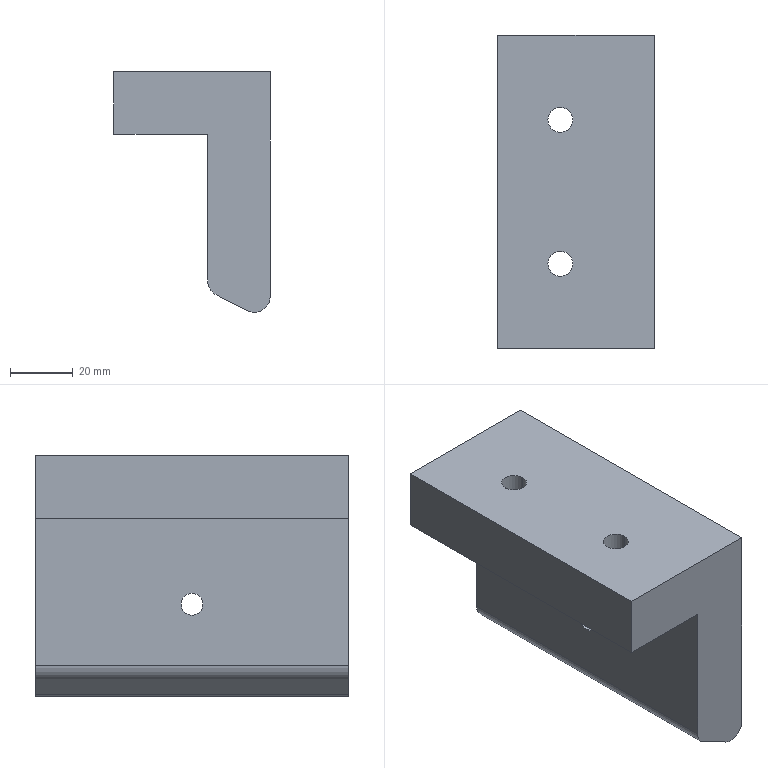Part | SolidWorks | features ICE 4, Extrusion 1, Fillet 1 | 1 solid | 23 faces | box 50 x 100 x 76.91 mm | volume 202541 mm3 | cylinder 13 | plane 10 | commonest cylinder face diameters 8 x4 16 x4 10 x3 7 x2
STEP:
#1=CARTESIAN_POINT('',(20.,100.,-66.91));
#2=VERTEX_POINT('',#1);
#3=CARTESIAN_POINT('',(17.764,100.,-66.382));
#4=VERTEX_POINT('',#3);
#5=CARTESIAN_POINT('',(20.,100.,-61.91));
#6=DIRECTION('',(0.,1.,0.));
#7=DIRECTION('',(0.,0.,1.));
#8=AXIS2_PLACEMENT_3D('',#5,#6,#7);
#9=CIRCLE('',#8,5.);
#10=EDGE_CURVE('',#2,#4,#9,.T.);
#11=ORIENTED_EDGE('',*,*,#10,.F.);
#12=CARTESIAN_POINT('',(20.,0.,-66.91));
#13=VERTEX_POINT('',#12);
#14=CARTESIAN_POINT('',(20.,-46.,-66.91));
#15=DIRECTION('',(0.,-1.,0.));
#16=VECTOR('',#15,1000.);
#17=LINE('',#14,#16);
#18=EDGE_CURVE('',#2,#13,#17,.T.);
#19=ORIENTED_EDGE('',*,*,#18,.T.);
#20=CARTESIAN_POINT('',(17.764,0.,-66.382));
#21=VERTEX_POINT('',#20);
#22=CARTESIAN_POINT('',(20.,0.,-61.91));
#23=DIRECTION('',(0.,-1.,0.));
#24=DIRECTION('',(0.,0.,1.));
#25=AXIS2_PLACEMENT_3D('',#22,#23,#24);
#26=CIRCLE('',#25,5.);
#27=EDGE_CURVE('',#21,#13,#26,.T.);
#28=ORIENTED_EDGE('',*,*,#27,.F.);
#29=CARTESIAN_POINT('',(17.764,-46.,-66.382));
#30=DIRECTION('',(0.,-1.,0.));
#31=VECTOR('',#30,1000.);
#32=LINE('',#29,#31);
#33=EDGE_CURVE('',#4,#21,#32,.T.);
#34=ORIENTED_EDGE('',*,*,#33,.F.);
#35=EDGE_LOOP('',(#11,#19,#28,#34));
#36=FACE_OUTER_BOUND('',#35,.T.);
#37=CARTESIAN_POINT('',(20.,-46.,-61.91));
#38=DIRECTION('',(0.,-1.,0.));
#39=DIRECTION('',(0.,0.,-1.));
#40=AXIS2_PLACEMENT_3D('',#37,#38,#39);
#41=CYLINDRICAL_SURFACE('',#40,5.);
#42=ADVANCED_FACE('',(#36),#41,.T.);
#43=CARTESIAN_POINT('',(3.,73.,0.));
#44=VERTEX_POINT('',#43);
#45=CARTESIAN_POINT('',(-13.,73.,0.));
#46=VERTEX_POINT('',#45);
#47=CARTESIAN_POINT('',(-5.,73.,0.));
#48=DIRECTION('',(0.,0.,-1.));
#49=DIRECTION('',(-1.,0.,0.));
#50=AXIS2_PLACEMENT_3D('',#47,#48,#49);
#51=CIRCLE('',#50,8.);
#52=EDGE_CURVE('',#44,#46,#51,.T.);
#53=ORIENTED_EDGE('',*,*,#52,.F.);
#54=CARTESIAN_POINT('',(3.,73.,-10.));
#55=VERTEX_POINT('',#54);
#56=CARTESIAN_POINT('',(3.,73.,0.));
#57=DIRECTION('',(0.,0.,-1.));
#58=VECTOR('',#57,1000.);
#59=LINE('',#56,#58);
#60=EDGE_CURVE('',#44,#55,#59,.T.);
#61=ORIENTED_EDGE('',*,*,#60,.T.);
#62=CARTESIAN_POINT('',(-13.,73.,-10.));
#63=VERTEX_POINT('',#62);
#64=CARTESIAN_POINT('',(-5.,73.,-10.));
#65=DIRECTION('',(0.,0.,-1.));
#66=DIRECTION('',(-1.,0.,0.));
#67=AXIS2_PLACEMENT_3D('',#64,#65,#66);
#68=CIRCLE('',#67,8.);
#69=EDGE_CURVE('',#55,#63,#68,.T.);
#70=ORIENTED_EDGE('',*,*,#69,.T.);
#71=CARTESIAN_POINT('',(-13.,73.,0.));
#72=DIRECTION('',(0.,0.,-1.));
#73=VECTOR('',#72,1000.);
#74=LINE('',#71,#73);
#75=EDGE_CURVE('',#46,#63,#74,.T.);
#76=ORIENTED_EDGE('',*,*,#75,.F.);
#77=EDGE_LOOP('',(#53,#61,#70,#76));
#78=FACE_OUTER_BOUND('',#77,.T.);
#79=CARTESIAN_POINT('',(-5.,73.,0.));
#80=DIRECTION('',(0.,0.,-1.));
#81=DIRECTION('',(-1.,0.,0.));
#82=AXIS2_PLACEMENT_3D('',#79,#80,#81);
#83=CYLINDRICAL_SURFACE('',#82,8.);
#84=ADVANCED_FACE('',(#78),#83,.F.);
#85=CARTESIAN_POINT('',(3.,27.,0.));
#86=VERTEX_POINT('',#85);
#87=CARTESIAN_POINT('',(-13.,27.,0.));
#88=VERTEX_POINT('',#87);
#89=CARTESIAN_POINT('',(-5.,27.,0.));
#90=DIRECTION('',(0.,0.,-1.));
#91=DIRECTION('',(-1.,0.,0.));
#92=AXIS2_PLACEMENT_3D('',#89,#90,#91);
#93=CIRCLE('',#92,8.);
#94=EDGE_CURVE('',#86,#88,#93,.T.);
#95=ORIENTED_EDGE('',*,*,#94,.F.);
#96=CARTESIAN_POINT('',(3.,27.,-10.));
#97=VERTEX_POINT('',#96);
#98=CARTESIAN_POINT('',(3.,27.,0.));
#99=DIRECTION('',(0.,0.,-1.));
#100=VECTOR('',#99,1000.);
#101=LINE('',#98,#100);
#102=EDGE_CURVE('',#86,#97,#101,.T.);
#103=ORIENTED_EDGE('',*,*,#102,.T.);
#104=CARTESIAN_POINT('',(-13.,27.,-10.));
#105=VERTEX_POINT('',#104);
#106=CARTESIAN_POINT('',(-5.,27.,-10.));
#107=DIRECTION('',(0.,0.,-1.));
#108=DIRECTION('',(-1.,0.,0.));
#109=AXIS2_PLACEMENT_3D('',#106,#107,#108);
#110=CIRCLE('',#109,8.);
#111=EDGE_CURVE('',#97,#105,#110,.T.);
#112=ORIENTED_EDGE('',*,*,#111,.T.);
#113=CARTESIAN_POINT('',(-13.,27.,0.));
#114=DIRECTION('',(0.,0.,-1.));
#115=VECTOR('',#114,1000.);
#116=LINE('',#113,#115);
#117=EDGE_CURVE('',#88,#105,#116,.T.);
#118=ORIENTED_EDGE('',*,*,#117,.F.);
#119=EDGE_LOOP('',(#95,#103,#112,#118));
#120=FACE_OUTER_BOUND('',#119,.T.);
#121=CARTESIAN_POINT('',(-5.,27.,0.));
#122=DIRECTION('',(0.,0.,-1.));
#123=DIRECTION('',(-1.,0.,0.));
#124=AXIS2_PLACEMENT_3D('',#121,#122,#123);
#125=CYLINDRICAL_SURFACE('',#124,8.);
#126=ADVANCED_FACE('',(#120),#125,.F.);
#127=CARTESIAN_POINT('',(25.,50.,-41.));
#128=VERTEX_POINT('',#127);
#129=CARTESIAN_POINT('',(25.,50.,-34.));
#130=VERTEX_POINT('',#129);
#131=CARTESIAN_POINT('',(25.,50.,-37.5));
#132=DIRECTION('',(-1.,0.,0.));
#133=DIRECTION('',(0.,0.,1.));
#134=AXIS2_PLACEMENT_3D('',#131,#132,#133);
#135=CIRCLE('',#134,3.5);
#136=EDGE_CURVE('',#128,#130,#135,.T.);
#137=ORIENTED_EDGE('',*,*,#136,.F.);
#138=CARTESIAN_POINT('',(5.,50.,-41.));
#139=VERTEX_POINT('',#138);
#140=CARTESIAN_POINT('',(105.,50.,-41.));
#141=DIRECTION('',(-1.,0.,0.));
#142=VECTOR('',#141,1000.);
#143=LINE('',#140,#142);
#144=EDGE_CURVE('',#128,#139,#143,.T.);
#145=ORIENTED_EDGE('',*,*,#144,.T.);
#146=CARTESIAN_POINT('',(5.,50.,-34.));
#147=VERTEX_POINT('',#146);
#148=CARTESIAN_POINT('',(5.,50.,-37.5));
#149=DIRECTION('',(-1.,0.,0.));
#150=DIRECTION('',(0.,0.,1.));
#151=AXIS2_PLACEMENT_3D('',#148,#149,#150);
#152=CIRCLE('',#151,3.5);
#153=EDGE_CURVE('',#139,#147,#152,.T.);
#154=ORIENTED_EDGE('',*,*,#153,.T.);
#155=CARTESIAN_POINT('',(105.,50.,-34.));
#156=DIRECTION('',(-1.,0.,0.));
#157=VECTOR('',#156,1000.);
#158=LINE('',#155,#157);
#159=EDGE_CURVE('',#130,#147,#158,.T.);
#160=ORIENTED_EDGE('',*,*,#159,.F.);
#161=EDGE_LOOP('',(#137,#145,#154,#160));
#162=FACE_OUTER_BOUND('',#161,.T.);
#163=CARTESIAN_POINT('',(105.,50.,-37.5));
#164=DIRECTION('',(-1.,0.,0.));
#165=DIRECTION('',(0.,0.,1.));
#166=AXIS2_PLACEMENT_3D('',#163,#164,#165);
#167=CYLINDRICAL_SURFACE('',#166,3.5);
#168=ADVANCED_FACE('',(#162),#167,.F.);
#169=CARTESIAN_POINT('',(-1.,27.,10.));
#170=VERTEX_POINT('',#169);
#171=CARTESIAN_POINT('',(-9.,27.,10.));
#172=VERTEX_POINT('',#171);
#173=CARTESIAN_POINT('',(-5.,27.,10.));
#174=DIRECTION('',(0.,0.,-1.));
#175=DIRECTION('',(-1.,0.,0.));
#176=AXIS2_PLACEMENT_3D('',#173,#174,#175);
#177=CIRCLE('',#176,4.);
#178=EDGE_CURVE('',#170,#172,#177,.T.);
#179=ORIENTED_EDGE('',*,*,#178,.F.);
#180=CARTESIAN_POINT('',(-1.,27.,0.));
#181=VERTEX_POINT('',#180);
#182=CARTESIAN_POINT('',(-1.,27.,90.));
#183=DIRECTION('',(0.,0.,-1.));
#184=VECTOR('',#183,1000.);
#185=LINE('',#182,#184);
#186=EDGE_CURVE('',#170,#181,#185,.T.);
#187=ORIENTED_EDGE('',*,*,#186,.T.);
#188=CARTESIAN_POINT('',(-9.,27.,0.));
#189=VERTEX_POINT('',#188);
#190=CARTESIAN_POINT('',(-5.,27.,0.));
#191=DIRECTION('',(0.,0.,1.));
#192=DIRECTION('',(-1.,0.,0.));
#193=AXIS2_PLACEMENT_3D('',#190,#191,#192);
#194=CIRCLE('',#193,4.);
#195=EDGE_CURVE('',#189,#181,#194,.T.);
#196=ORIENTED_EDGE('',*,*,#195,.F.);
#197=CARTESIAN_POINT('',(-9.,27.,90.));
#198=DIRECTION('',(0.,0.,-1.));
#199=VECTOR('',#198,1000.);
#200=LINE('',#197,#199);
#201=EDGE_CURVE('',#172,#189,#200,.T.);
#202=ORIENTED_EDGE('',*,*,#201,.F.);
#203=EDGE_LOOP('',(#179,#187,#196,#202));
#204=FACE_OUTER_BOUND('',#203,.T.);
#205=CARTESIAN_POINT('',(-5.,27.,90.));
#206=DIRECTION('',(0.,0.,-1.));
#207=DIRECTION('',(-1.,0.,0.));
#208=AXIS2_PLACEMENT_3D('',#205,#206,#207);
#209=CYLINDRICAL_SURFACE('',#208,4.);
#210=ADVANCED_FACE('',(#204),#209,.F.);
#211=CARTESIAN_POINT('',(-1.,73.,10.));
#212=VERTEX_POINT('',#211);
#213=CARTESIAN_POINT('',(-9.,73.,10.));
#214=VERTEX_POINT('',#213);
#215=CARTESIAN_POINT('',(-5.,73.,10.));
#216=DIRECTION('',(0.,0.,-1.));
#217=DIRECTION('',(-1.,0.,0.));
#218=AXIS2_PLACEMENT_3D('',#215,#216,#217);
#219=CIRCLE('',#218,4.);
#220=EDGE_CURVE('',#212,#214,#219,.T.);
#221=ORIENTED_EDGE('',*,*,#220,.F.);
#222=CARTESIAN_POINT('',(-1.,73.,0.));
#223=VERTEX_POINT('',#222);
#224=CARTESIAN_POINT('',(-1.,73.,90.));
#225=DIRECTION('',(0.,0.,-1.));
#226=VECTOR('',#225,1000.);
#227=LINE('',#224,#226);
#228=EDGE_CURVE('',#212,#223,#227,.T.);
#229=ORIENTED_EDGE('',*,*,#228,.T.);
#230=CARTESIAN_POINT('',(-9.,73.,0.));
#231=VERTEX_POINT('',#230);
#232=CARTESIAN_POINT('',(-5.,73.,0.));
#233=DIRECTION('',(0.,0.,1.));
#234=DIRECTION('',(-1.,0.,0.));
#235=AXIS2_PLACEMENT_3D('',#232,#233,#234);
#236=CIRCLE('',#235,4.);
#237=EDGE_CURVE('',#231,#223,#236,.T.);
#238=ORIENTED_EDGE('',*,*,#237,.F.);
#239=CARTESIAN_POINT('',(-9.,73.,90.));
#240=DIRECTION('',(0.,0.,-1.));
#241=VECTOR('',#240,1000.);
#242=LINE('',#239,#241);
#243=EDGE_CURVE('',#214,#231,#242,.T.);
#244=ORIENTED_EDGE('',*,*,#243,.F.);
#245=EDGE_LOOP('',(#221,#229,#238,#244));
#246=FACE_OUTER_BOUND('',#245,.T.);
#247=CARTESIAN_POINT('',(-5.,73.,90.));
#248=DIRECTION('',(0.,0.,-1.));
#249=DIRECTION('',(-1.,0.,0.));
#250=AXIS2_PLACEMENT_3D('',#247,#248,#249);
#251=CYLINDRICAL_SURFACE('',#250,4.);
#252=ADVANCED_FACE('',(#246),#251,.F.);
#253=ORIENTED_EDGE('',*,*,#228,.F.);
#254=CARTESIAN_POINT('',(-5.,73.,10.));
#255=DIRECTION('',(0.,0.,-1.));
#256=DIRECTION('',(-1.,0.,0.));
#257=AXIS2_PLACEMENT_3D('',#254,#255,#256);
#258=CIRCLE('',#257,4.);
#259=EDGE_CURVE('',#214,#212,#258,.T.);
#260=ORIENTED_EDGE('',*,*,#259,.F.);
#261=ORIENTED_EDGE('',*,*,#243,.T.);
#262=CARTESIAN_POINT('',(-5.,73.,0.));
#263=DIRECTION('',(0.,0.,1.));
#264=DIRECTION('',(-1.,0.,0.));
#265=AXIS2_PLACEMENT_3D('',#262,#263,#264);
#266=CIRCLE('',#265,4.);
#267=EDGE_CURVE('',#223,#231,#266,.T.);
#268=ORIENTED_EDGE('',*,*,#267,.F.);
#269=EDGE_LOOP('',(#253,#260,#261,#268));
#270=FACE_OUTER_BOUND('',#269,.T.);
#271=CARTESIAN_POINT('',(-5.,73.,90.));
#272=DIRECTION('',(0.,0.,-1.));
#273=DIRECTION('',(-1.,0.,0.));
#274=AXIS2_PLACEMENT_3D('',#271,#272,#273);
#275=CYLINDRICAL_SURFACE('',#274,4.);
#276=ADVANCED_FACE('',(#270),#275,.F.);
#277=ORIENTED_EDGE('',*,*,#186,.F.);
#278=CARTESIAN_POINT('',(-5.,27.,10.));
#279=DIRECTION('',(0.,0.,-1.));
#280=DIRECTION('',(-1.,0.,0.));
#281=AXIS2_PLACEMENT_3D('',#278,#279,#280);
#282=CIRCLE('',#281,4.);
#283=EDGE_CURVE('',#172,#170,#282,.T.);
#284=ORIENTED_EDGE('',*,*,#283,.F.);
#285=ORIENTED_EDGE('',*,*,#201,.T.);
#286=CARTESIAN_POINT('',(-5.,27.,0.));
#287=DIRECTION('',(0.,0.,1.));
#288=DIRECTION('',(-1.,0.,0.));
#289=AXIS2_PLACEMENT_3D('',#286,#287,#288);
#290=CIRCLE('',#289,4.);
#291=EDGE_CURVE('',#181,#189,#290,.T.);
#292=ORIENTED_EDGE('',*,*,#291,.F.);
#293=EDGE_LOOP('',(#277,#284,#285,#292));
#294=FACE_OUTER_BOUND('',#293,.T.);
#295=CARTESIAN_POINT('',(-5.,27.,90.));
#296=DIRECTION('',(0.,0.,-1.));
#297=DIRECTION('',(-1.,0.,0.));
#298=AXIS2_PLACEMENT_3D('',#295,#296,#297);
#299=CYLINDRICAL_SURFACE('',#298,4.);
#300=ADVANCED_FACE('',(#294),#299,.F.);
#301=CARTESIAN_POINT('',(25.,50.,-37.5));
#302=DIRECTION('',(-1.,0.,0.));
#303=DIRECTION('',(0.,0.,1.));
#304=AXIS2_PLACEMENT_3D('',#301,#302,#303);
#305=CIRCLE('',#304,3.5);
#306=EDGE_CURVE('',#130,#128,#305,.T.);
#307=ORIENTED_EDGE('',*,*,#306,.T.);
#308=ORIENTED_EDGE('',*,*,#136,.T.);
#309=EDGE_LOOP('',(#307,#308));
#310=FACE_BOUND('',#309,.T.);
#311=CARTESIAN_POINT('',(25.,0.,10.));
#312=VERTEX_POINT('',#311);
#313=CARTESIAN_POINT('',(25.,0.,-61.91));
#314=VERTEX_POINT('',#313);
#315=CARTESIAN_POINT('',(25.,0.,0.));
#316=DIRECTION('',(0.,0.,-1.));
#317=VECTOR('',#316,1000.);
#318=LINE('',#315,#317);
#319=EDGE_CURVE('',#312,#314,#318,.T.);
#320=ORIENTED_EDGE('',*,*,#319,.T.);
#321=CARTESIAN_POINT('',(25.,100.,-61.91));
#322=VERTEX_POINT('',#321);
#323=CARTESIAN_POINT('',(25.,100.,-61.91));
#324=DIRECTION('',(0.,1.,0.));
#325=VECTOR('',#324,1000.);
#326=LINE('',#323,#325);
#327=EDGE_CURVE('',#314,#322,#326,.T.);
#328=ORIENTED_EDGE('',*,*,#327,.T.);
#329=CARTESIAN_POINT('',(25.,100.,10.));
#330=VERTEX_POINT('',#329);
#331=CARTESIAN_POINT('',(25.,100.,0.));
#332=DIRECTION('',(0.,0.,-1.));
#333=VECTOR('',#332,1000.);
#334=LINE('',#331,#333);
#335=EDGE_CURVE('',#330,#322,#334,.T.);
#336=ORIENTED_EDGE('',*,*,#335,.F.);
#337=CARTESIAN_POINT('',(25.,100.,10.));
#338=DIRECTION('',(0.,-1.,0.));
#339=VECTOR('',#338,1000.);
#340=LINE('',#337,#339);
#341=EDGE_CURVE('',#330,#312,#340,.T.);
#342=ORIENTED_EDGE('',*,*,#341,.T.);
#343=EDGE_LOOP('',(#320,#328,#336,#342));
#344=FACE_OUTER_BOUND('',#343,.T.);
#345=CARTESIAN_POINT('',(25.,100.,0.));
#346=DIRECTION('',(-1.,0.,0.));
#347=DIRECTION('',(0.,0.,1.));
#348=AXIS2_PLACEMENT_3D('',#345,#346,#347);
#349=PLANE('',#348);
#350=ADVANCED_FACE('',(#310,#344),#349,.F.);
#351=CARTESIAN_POINT('',(5.,100.,-10.));
#352=VERTEX_POINT('',#351);
#353=CARTESIAN_POINT('',(5.,100.,-56.91));
#354=VERTEX_POINT('',#353);
#355=CARTESIAN_POINT('',(5.,100.,0.));
#356=DIRECTION('',(0.,0.,-1.));
#357=VECTOR('',#356,1000.);
#358=LINE('',#355,#357);
#359=EDGE_CURVE('',#352,#354,#358,.T.);
#360=ORIENTED_EDGE('',*,*,#359,.T.);
#361=CARTESIAN_POINT('',(5.,0.,-56.91));
#362=VERTEX_POINT('',#361);
#363=CARTESIAN_POINT('',(5.,0.,-56.91));
#364=DIRECTION('',(0.,-1.,0.));
#365=VECTOR('',#364,1000.);
#366=LINE('',#363,#365);
#367=EDGE_CURVE('',#354,#362,#366,.T.);
#368=ORIENTED_EDGE('',*,*,#367,.T.);
#369=CARTESIAN_POINT('',(5.,0.,-10.));
#370=VERTEX_POINT('',#369);
#371=CARTESIAN_POINT('',(5.,0.,0.));
#372=DIRECTION('',(0.,0.,-1.));
#373=VECTOR('',#372,1000.);
#374=LINE('',#371,#373);
#375=EDGE_CURVE('',#370,#362,#374,.T.);
#376=ORIENTED_EDGE('',*,*,#375,.F.);
#377=CARTESIAN_POINT('',(5.,100.,-10.));
#378=DIRECTION('',(0.,-1.,0.));
#379=VECTOR('',#378,1000.);
#380=LINE('',#377,#379);
#381=EDGE_CURVE('',#352,#370,#380,.T.);
#382=ORIENTED_EDGE('',*,*,#381,.F.);
#383=EDGE_LOOP('',(#360,#368,#376,#382));
#384=FACE_OUTER_BOUND('',#383,.T.);
#385=CARTESIAN_POINT('',(5.,50.,-37.5));
#386=DIRECTION('',(-1.,0.,0.));
#387=DIRECTION('',(0.,0.,1.));
#388=AXIS2_PLACEMENT_3D('',#385,#386,#387);
#389=CIRCLE('',#388,3.5);
#390=EDGE_CURVE('',#147,#139,#389,.T.);
#391=ORIENTED_EDGE('',*,*,#390,.F.);
#392=ORIENTED_EDGE('',*,*,#153,.F.);
#393=EDGE_LOOP('',(#391,#392));
#394=FACE_BOUND('',#393,.T.);
#395=CARTESIAN_POINT('',(5.,100.,0.));
#396=DIRECTION('',(-1.,0.,0.));
#397=DIRECTION('',(0.,0.,1.));
#398=AXIS2_PLACEMENT_3D('',#395,#396,#397);
#399=PLANE('',#398);
#400=ADVANCED_FACE('',(#384,#394),#399,.T.);
#401=CARTESIAN_POINT('',(-5.,27.,-10.));
#402=DIRECTION('',(0.,0.,-1.));
#403=DIRECTION('',(-1.,0.,0.));
#404=AXIS2_PLACEMENT_3D('',#401,#402,#403);
#405=CIRCLE('',#404,8.);
#406=EDGE_CURVE('',#105,#97,#405,.T.);
#407=ORIENTED_EDGE('',*,*,#406,.F.);
#408=ORIENTED_EDGE('',*,*,#111,.F.);
#409=EDGE_LOOP('',(#407,#408));
#410=FACE_BOUND('',#409,.T.);
#411=CARTESIAN_POINT('',(-5.,73.,-10.));
#412=DIRECTION('',(0.,0.,-1.));
#413=DIRECTION('',(-1.,0.,0.));
#414=AXIS2_PLACEMENT_3D('',#411,#412,#413);
#415=CIRCLE('',#414,8.);
#416=EDGE_CURVE('',#63,#55,#415,.T.);
#417=ORIENTED_EDGE('',*,*,#416,.F.);
#418=ORIENTED_EDGE('',*,*,#69,.F.);
#419=EDGE_LOOP('',(#417,#418));
#420=FACE_BOUND('',#419,.T.);
#421=CARTESIAN_POINT('',(-25.,0.,-10.));
#422=VERTEX_POINT('',#421);
#423=CARTESIAN_POINT('',(0.,0.,-10.));
#424=DIRECTION('',(1.,0.,0.));
#425=VECTOR('',#424,1000.);
#426=LINE('',#423,#425);
#427=EDGE_CURVE('',#422,#370,#426,.T.);
#428=ORIENTED_EDGE('',*,*,#427,.F.);
#429=CARTESIAN_POINT('',(-25.,100.,-10.));
#430=VERTEX_POINT('',#429);
#431=CARTESIAN_POINT('',(-25.,100.,-10.));
#432=DIRECTION('',(0.,-1.,0.));
#433=VECTOR('',#432,1000.);
#434=LINE('',#431,#433);
#435=EDGE_CURVE('',#430,#422,#434,.T.);
#436=ORIENTED_EDGE('',*,*,#435,.F.);
#437=CARTESIAN_POINT('',(0.,100.,-10.));
#438=DIRECTION('',(1.,0.,0.));
#439=VECTOR('',#438,1000.);
#440=LINE('',#437,#439);
#441=EDGE_CURVE('',#430,#352,#440,.T.);
#442=ORIENTED_EDGE('',*,*,#441,.T.);
#443=ORIENTED_EDGE('',*,*,#381,.T.);
#444=EDGE_LOOP('',(#428,#436,#442,#443));
#445=FACE_OUTER_BOUND('',#444,.T.);
#446=CARTESIAN_POINT('',(0.,100.,-10.));
#447=DIRECTION('',(0.,0.,-1.));
#448=DIRECTION('',(-1.,0.,0.));
#449=AXIS2_PLACEMENT_3D('',#446,#447,#448);
#450=PLANE('',#449);
#451=ADVANCED_FACE('',(#410,#420,#445),#450,.T.);
#452=CARTESIAN_POINT('',(-25.,0.,10.));
#453=VERTEX_POINT('',#452);
#454=CARTESIAN_POINT('',(-25.,0.,0.));
#455=DIRECTION('',(0.,0.,-1.));
#456=VECTOR('',#455,1000.);
#457=LINE('',#454,#456);
#458=EDGE_CURVE('',#453,#422,#457,.T.);
#459=ORIENTED_EDGE('',*,*,#458,.F.);
#460=CARTESIAN_POINT('',(-25.,100.,10.));
#461=VERTEX_POINT('',#460);
#462=CARTESIAN_POINT('',(-25.,100.,10.));
#463=DIRECTION('',(0.,-1.,0.));
#464=VECTOR('',#463,1000.);
#465=LINE('',#462,#464);
#466=EDGE_CURVE('',#461,#453,#465,.T.);
#467=ORIENTED_EDGE('',*,*,#466,.F.);
#468=CARTESIAN_POINT('',(-25.,100.,0.));
#469=DIRECTION('',(0.,0.,-1.));
#470=VECTOR('',#469,1000.);
#471=LINE('',#468,#470);
#472=EDGE_CURVE('',#461,#430,#471,.T.);
#473=ORIENTED_EDGE('',*,*,#472,.T.);
#474=ORIENTED_EDGE('',*,*,#435,.T.);
#475=EDGE_LOOP('',(#459,#467,#473,#474));
#476=FACE_OUTER_BOUND('',#475,.T.);
#477=CARTESIAN_POINT('',(-25.,100.,0.));
#478=DIRECTION('',(-1.,0.,0.));
#479=DIRECTION('',(0.,0.,1.));
#480=AXIS2_PLACEMENT_3D('',#477,#478,#479);
#481=PLANE('',#480);
#482=ADVANCED_FACE('',(#476),#481,.T.);
#483=ORIENTED_EDGE('',*,*,#283,.T.);
#484=ORIENTED_EDGE('',*,*,#178,.T.);
#485=EDGE_LOOP('',(#483,#484));
#486=FACE_BOUND('',#485,.T.);
#487=ORIENTED_EDGE('',*,*,#259,.T.);
#488=ORIENTED_EDGE('',*,*,#220,.T.);
#489=EDGE_LOOP('',(#487,#488));
#490=FACE_BOUND('',#489,.T.);
#491=CARTESIAN_POINT('',(0.,0.,10.));
#492=DIRECTION('',(1.,0.,0.));
#493=VECTOR('',#492,1000.);
#494=LINE('',#491,#493);
#495=EDGE_CURVE('',#453,#312,#494,.T.);
#496=ORIENTED_EDGE('',*,*,#495,.T.);
#497=ORIENTED_EDGE('',*,*,#341,.F.);
#498=CARTESIAN_POINT('',(0.,100.,10.));
#499=DIRECTION('',(1.,0.,0.));
#500=VECTOR('',#499,1000.);
#501=LINE('',#498,#500);
#502=EDGE_CURVE('',#461,#330,#501,.T.);
#503=ORIENTED_EDGE('',*,*,#502,.F.);
#504=ORIENTED_EDGE('',*,*,#466,.T.);
#505=EDGE_LOOP('',(#496,#497,#503,#504));
#506=FACE_OUTER_BOUND('',#505,.T.);
#507=CARTESIAN_POINT('',(0.,100.,10.));
#508=DIRECTION('',(0.,0.,-1.));
#509=DIRECTION('',(-1.,0.,0.));
#510=AXIS2_PLACEMENT_3D('',#507,#508,#509);
#511=PLANE('',#510);
#512=ADVANCED_FACE('',(#486,#490,#506),#511,.F.);
#513=ORIENTED_EDGE('',*,*,#335,.T.);
#514=CARTESIAN_POINT('',(20.,100.,-61.91));
#515=DIRECTION('',(0.,1.,0.));
#516=DIRECTION('',(0.,0.,1.));
#517=AXIS2_PLACEMENT_3D('',#514,#515,#516);
#518=CIRCLE('',#517,5.);
#519=EDGE_CURVE('',#322,#2,#518,.T.);
#520=ORIENTED_EDGE('',*,*,#519,.T.);
#521=ORIENTED_EDGE('',*,*,#10,.T.);
#522=CARTESIAN_POINT('',(7.764,100.,-61.382));
#523=VERTEX_POINT('',#522);
#524=CARTESIAN_POINT('',(5.,100.,-60.));
#525=DIRECTION('',(0.8944,0.,-0.4472));
#526=VECTOR('',#525,1000.);
#527=LINE('',#524,#526);
#528=EDGE_CURVE('',#523,#4,#527,.T.);
#529=ORIENTED_EDGE('',*,*,#528,.F.);
#530=CARTESIAN_POINT('',(10.,100.,-56.91));
#531=DIRECTION('',(0.,1.,0.));
#532=DIRECTION('',(0.,0.,1.));
#533=AXIS2_PLACEMENT_3D('',#530,#531,#532);
#534=CIRCLE('',#533,5.);
#535=EDGE_CURVE('',#523,#354,#534,.T.);
#536=ORIENTED_EDGE('',*,*,#535,.T.);
#537=ORIENTED_EDGE('',*,*,#359,.F.);
#538=ORIENTED_EDGE('',*,*,#441,.F.);
#539=ORIENTED_EDGE('',*,*,#472,.F.);
#540=ORIENTED_EDGE('',*,*,#502,.T.);
#541=EDGE_LOOP('',(#513,#520,#521,#529,#536,#537,#538,#539,#540));
#542=FACE_OUTER_BOUND('',#541,.T.);
#543=CARTESIAN_POINT('',(0.,100.,0.));
#544=DIRECTION('',(0.,1.,0.));
#545=DIRECTION('',(0.,0.,1.));
#546=AXIS2_PLACEMENT_3D('',#543,#544,#545);
#547=PLANE('',#546);
#548=ADVANCED_FACE('',(#542),#547,.T.);
#549=CARTESIAN_POINT('',(7.764,0.,-61.382));
#550=VERTEX_POINT('',#549);
#551=CARTESIAN_POINT('',(-23.,0.,-46.));
#552=DIRECTION('',(0.8944,0.,-0.4472));
#553=VECTOR('',#552,1000.);
#554=LINE('',#551,#553);
#555=EDGE_CURVE('',#550,#21,#554,.T.);
#556=ORIENTED_EDGE('',*,*,#555,.T.);
#557=ORIENTED_EDGE('',*,*,#27,.T.);
#558=CARTESIAN_POINT('',(20.,0.,-61.91));
#559=DIRECTION('',(0.,-1.,0.));
#560=DIRECTION('',(0.,0.,1.));
#561=AXIS2_PLACEMENT_3D('',#558,#559,#560);
#562=CIRCLE('',#561,5.);
#563=EDGE_CURVE('',#13,#314,#562,.T.);
#564=ORIENTED_EDGE('',*,*,#563,.T.);
#565=ORIENTED_EDGE('',*,*,#319,.F.);
#566=ORIENTED_EDGE('',*,*,#495,.F.);
#567=ORIENTED_EDGE('',*,*,#458,.T.);
#568=ORIENTED_EDGE('',*,*,#427,.T.);
#569=ORIENTED_EDGE('',*,*,#375,.T.);
#570=CARTESIAN_POINT('',(10.,0.,-56.91));
#571=DIRECTION('',(0.,-1.,0.));
#572=DIRECTION('',(0.,0.,1.));
#573=AXIS2_PLACEMENT_3D('',#570,#571,#572);
#574=CIRCLE('',#573,5.);
#575=EDGE_CURVE('',#362,#550,#574,.T.);
#576=ORIENTED_EDGE('',*,*,#575,.T.);
#577=EDGE_LOOP('',(#556,#557,#564,#565,#566,#567,#568,#569,#576));
#578=FACE_OUTER_BOUND('',#577,.T.);
#579=CARTESIAN_POINT('',(0.,0.,0.));
#580=DIRECTION('',(0.,1.,0.));
#581=DIRECTION('',(0.,0.,1.));
#582=AXIS2_PLACEMENT_3D('',#579,#580,#581);
#583=PLANE('',#582);
#584=ADVANCED_FACE('',(#578),#583,.F.);
#585=ORIENTED_EDGE('',*,*,#144,.F.);
#586=ORIENTED_EDGE('',*,*,#306,.F.);
#587=ORIENTED_EDGE('',*,*,#159,.T.);
#588=ORIENTED_EDGE('',*,*,#390,.T.);
#589=EDGE_LOOP('',(#585,#586,#587,#588));
#590=FACE_OUTER_BOUND('',#589,.T.);
#591=CARTESIAN_POINT('',(105.,50.,-37.5));
#592=DIRECTION('',(-1.,0.,0.));
#593=DIRECTION('',(0.,0.,1.));
#594=AXIS2_PLACEMENT_3D('',#591,#592,#593);
#595=CYLINDRICAL_SURFACE('',#594,3.5);
#596=ADVANCED_FACE('',(#590),#595,.F.);
#597=CARTESIAN_POINT('',(-5.,27.,0.));
#598=DIRECTION('',(0.,0.,-1.));
#599=DIRECTION('',(-1.,0.,0.));
#600=AXIS2_PLACEMENT_3D('',#597,#598,#599);
#601=CIRCLE('',#600,8.);
#602=EDGE_CURVE('',#88,#86,#601,.T.);
#603=ORIENTED_EDGE('',*,*,#602,.T.);
#604=ORIENTED_EDGE('',*,*,#94,.T.);
#605=EDGE_LOOP('',(#603,#604));
#606=FACE_OUTER_BOUND('',#605,.T.);
#607=ORIENTED_EDGE('',*,*,#195,.T.);
#608=ORIENTED_EDGE('',*,*,#291,.T.);
#609=EDGE_LOOP('',(#607,#608));
#610=FACE_BOUND('',#609,.T.);
#611=CARTESIAN_POINT('',(-5.,27.,0.));
#612=DIRECTION('',(0.,0.,-1.));
#613=DIRECTION('',(-1.,0.,0.));
#614=AXIS2_PLACEMENT_3D('',#611,#612,#613);
#615=PLANE('',#614);
#616=ADVANCED_FACE('',(#606,#610),#615,.T.);
#617=ORIENTED_EDGE('',*,*,#102,.F.);
#618=ORIENTED_EDGE('',*,*,#602,.F.);
#619=ORIENTED_EDGE('',*,*,#117,.T.);
#620=ORIENTED_EDGE('',*,*,#406,.T.);
#621=EDGE_LOOP('',(#617,#618,#619,#620));
#622=FACE_OUTER_BOUND('',#621,.T.);
#623=CARTESIAN_POINT('',(-5.,27.,0.));
#624=DIRECTION('',(0.,0.,-1.));
#625=DIRECTION('',(-1.,0.,0.));
#626=AXIS2_PLACEMENT_3D('',#623,#624,#625);
#627=CYLINDRICAL_SURFACE('',#626,8.);
#628=ADVANCED_FACE('',(#622),#627,.F.);
#629=CARTESIAN_POINT('',(-5.,73.,0.));
#630=DIRECTION('',(0.,0.,-1.));
#631=DIRECTION('',(-1.,0.,0.));
#632=AXIS2_PLACEMENT_3D('',#629,#630,#631);
#633=CIRCLE('',#632,8.);
#634=EDGE_CURVE('',#46,#44,#633,.T.);
#635=ORIENTED_EDGE('',*,*,#634,.T.);
#636=ORIENTED_EDGE('',*,*,#52,.T.);
#637=EDGE_LOOP('',(#635,#636));
#638=FACE_OUTER_BOUND('',#637,.T.);
#639=ORIENTED_EDGE('',*,*,#237,.T.);
#640=ORIENTED_EDGE('',*,*,#267,.T.);
#641=EDGE_LOOP('',(#639,#640));
#642=FACE_BOUND('',#641,.T.);
#643=CARTESIAN_POINT('',(-5.,73.,0.));
#644=DIRECTION('',(0.,0.,-1.));
#645=DIRECTION('',(-1.,0.,0.));
#646=AXIS2_PLACEMENT_3D('',#643,#644,#645);
#647=PLANE('',#646);
#648=ADVANCED_FACE('',(#638,#642),#647,.T.);
#649=ORIENTED_EDGE('',*,*,#60,.F.);
#650=ORIENTED_EDGE('',*,*,#634,.F.);
#651=ORIENTED_EDGE('',*,*,#75,.T.);
#652=ORIENTED_EDGE('',*,*,#416,.T.);
#653=EDGE_LOOP('',(#649,#650,#651,#652));
#654=FACE_OUTER_BOUND('',#653,.T.);
#655=CARTESIAN_POINT('',(-5.,73.,0.));
#656=DIRECTION('',(0.,0.,-1.));
#657=DIRECTION('',(-1.,0.,0.));
#658=AXIS2_PLACEMENT_3D('',#655,#656,#657);
#659=CYLINDRICAL_SURFACE('',#658,8.);
#660=ADVANCED_FACE('',(#654),#659,.F.);
#661=ORIENTED_EDGE('',*,*,#528,.T.);
#662=ORIENTED_EDGE('',*,*,#33,.T.);
#663=ORIENTED_EDGE('',*,*,#555,.F.);
#664=CARTESIAN_POINT('',(7.764,100.,-61.382));
#665=DIRECTION('',(0.,1.,0.));
#666=VECTOR('',#665,1000.);
#667=LINE('',#664,#666);
#668=EDGE_CURVE('',#550,#523,#667,.T.);
#669=ORIENTED_EDGE('',*,*,#668,.T.);
#670=EDGE_LOOP('',(#661,#662,#663,#669));
#671=FACE_OUTER_BOUND('',#670,.T.);
#672=CARTESIAN_POINT('',(5.,-46.,-60.));
#673=DIRECTION('',(0.4472,0.,0.8944));
#674=DIRECTION('',(0.8944,0.,-0.4472));
#675=AXIS2_PLACEMENT_3D('',#672,#673,#674);
#676=PLANE('',#675);
#677=ADVANCED_FACE('',(#671),#676,.F.);
#678=ORIENTED_EDGE('',*,*,#18,.F.);
#679=ORIENTED_EDGE('',*,*,#519,.F.);
#680=ORIENTED_EDGE('',*,*,#327,.F.);
#681=ORIENTED_EDGE('',*,*,#563,.F.);
#682=EDGE_LOOP('',(#678,#679,#680,#681));
#683=FACE_OUTER_BOUND('',#682,.T.);
#684=CARTESIAN_POINT('',(20.,-46.,-61.91));
#685=DIRECTION('',(0.,-1.,0.));
#686=DIRECTION('',(0.,0.,-1.));
#687=AXIS2_PLACEMENT_3D('',#684,#685,#686);
#688=CYLINDRICAL_SURFACE('',#687,5.);
#689=ADVANCED_FACE('',(#683),#688,.T.);
#690=ORIENTED_EDGE('',*,*,#575,.F.);
#691=ORIENTED_EDGE('',*,*,#367,.F.);
#692=ORIENTED_EDGE('',*,*,#535,.F.);
#693=ORIENTED_EDGE('',*,*,#668,.F.);
#694=EDGE_LOOP('',(#690,#691,#692,#693));
#695=FACE_OUTER_BOUND('',#694,.T.);
#696=CARTESIAN_POINT('',(10.,-46.,-56.91));
#697=DIRECTION('',(0.,-1.,0.));
#698=DIRECTION('',(0.,0.,-1.));
#699=AXIS2_PLACEMENT_3D('',#696,#697,#698);
#700=CYLINDRICAL_SURFACE('',#699,5.);
#701=ADVANCED_FACE('',(#695),#700,.T.);
#702=CLOSED_SHELL('',(#42,#84,#126,#168,#210,#252,#276,#300,#350,#400,#451,#482,#512,#548,#584,#596,#616,#628,#648,#660,#677,#689,#701));
#703=MANIFOLD_SOLID_BREP('',#702);
#704=CARTESIAN_POINT('',(0.,0.,0.));
#705=DIRECTION('',(0.,0.,1.));
#706=DIRECTION('',(1.,0.,0.));
#707=AXIS2_PLACEMENT_3D('',#704,#705,#706);
#708=(LENGTH_UNIT()NAMED_UNIT(*)SI_UNIT(.MILLI.,.METRE.));
#709=UNCERTAINTY_MEASURE_WITH_UNIT(LENGTH_MEASURE(0.00001),#708,'','');
#710=(NAMED_UNIT(*)PLANE_ANGLE_UNIT()SI_UNIT($,.RADIAN.));
#711=(NAMED_UNIT(*)SI_UNIT($,.STERADIAN.)SOLID_ANGLE_UNIT());
#712=(GEOMETRIC_REPRESENTATION_CONTEXT(3)GLOBAL_UNCERTAINTY_ASSIGNED_CONTEXT((#709))GLOBAL_UNIT_ASSIGNED_CONTEXT((#708,#710,#711))REPRESENTATION_CONTEXT('',''));
#713=ADVANCED_BREP_SHAPE_REPRESENTATION('',(#703,#707),#712);